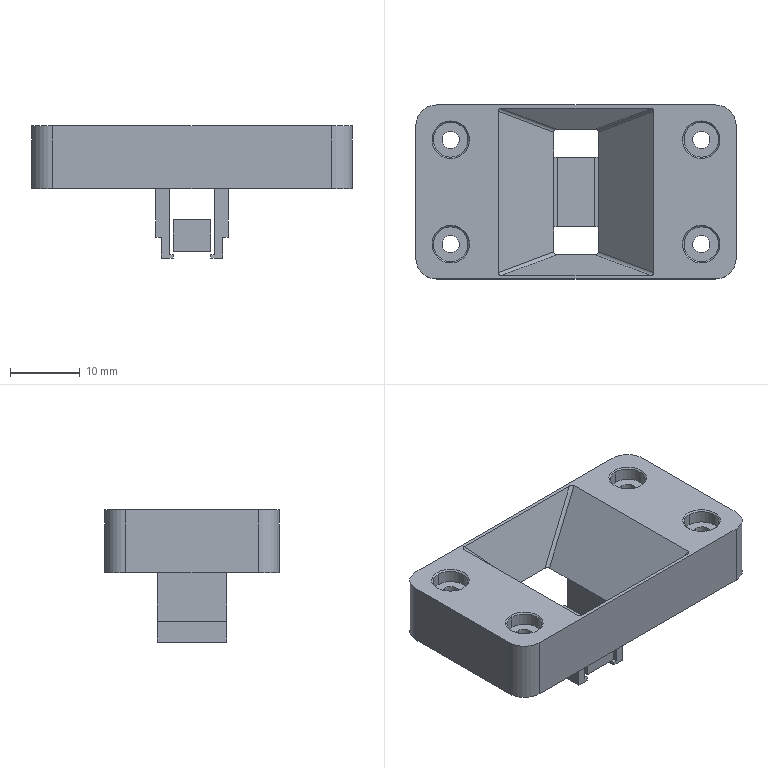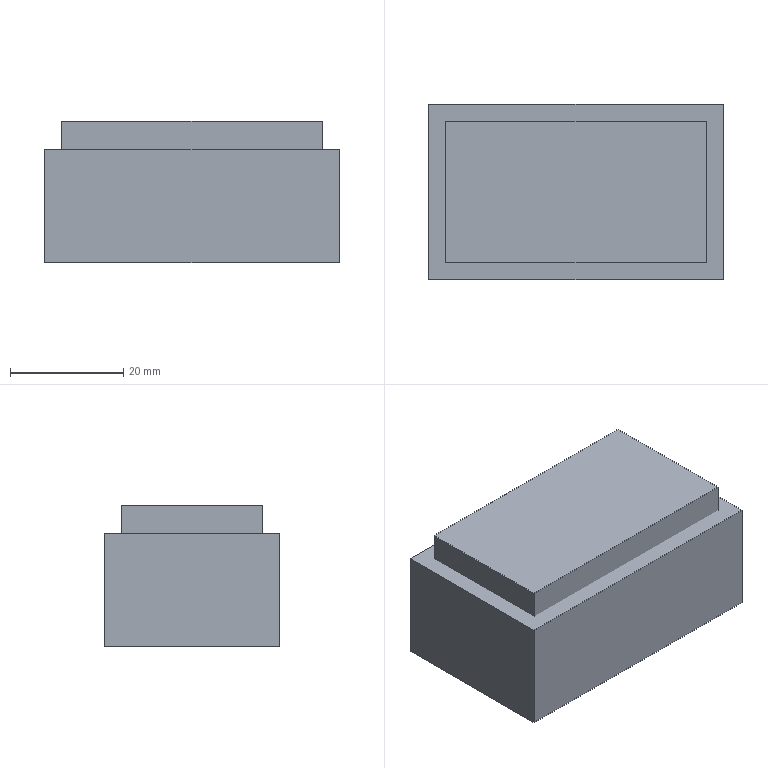CAM job | NX | 3-axis milling, drilling | part box 46 x 25 x 19 mm | stock box 52 x 31 x 25 mm
Tools:
number,name,description,diameter,corner_radius,flute_length,length,flutes
1,D63,Milling Tool-5 Parameters,63.0,0.0,50.0,75.0,2
7,D6A45,Milling Tool-5 Parameters,6.0,0.0,3.0,3.0,2
12,2.5ZT,Drilling Tool,2.5,0.0,35.0,50.0,2
10,D10,Milling Tool-5 Parameters,10.0,0.0,50.0,75.0,2
11,D10JING,Milling Tool-5 Parameters,10.0,0.0,50.0,75.0,2
3,D3,Milling Tool-5 Parameters,3.0,0.0,50.0,75.0,2
6,D6,Milling Tool-5 Parameters,6.0,0.0,50.0,75.0,2
4,D4,Milling Tool-5 Parameters,4.0,0.0,50.0,75.0,2
5,D2R0.2,Milling Tool-5 Parameters,2.0,0.2,50.0,75.0,2
Operations:
program,operation,operation_type,tool,method,geometry_group,spindle_rpm,surface_speed,feed_per_tooth,feed_cut,feed_plunge,cut_length_mm,path_length_mm,cut_time_min,machine_time_min
1,FLOOR_WALL,VolumeBased25DMillingOperation,D63,METHOD,A,6500.0,1286.0,0.0962,1250.0,100.0,127.0,181.0,0.1016,0.107
1,DRILLING_COPY_1,Operation,D6A45,METHOD,A,5000.0,94.0,0.025,250.0,0.0,16.0,167.719,0.064,0.0792
1,DRILLING_COPY_COPY_1,Operation,2.5ZT,METHOD,A,2000.0,15.0,0.03,120.0,0.0,57.004,252.718,0.475,0.4946
1,ADAPTIVE_MILLING,CavityMilling,D10,METHOD,A,9500.0,298.0,0.1579,3000.0,1000.0,710.321,804.321,0.2374,0.2468
1,ZLEVEL_PROFILE_COPY_COPY_1,ZLevelMilling,D10JING,METHOD,A,9500.0,298.0,0.0632,1200.0,100.0,176.311,268.311,0.1469,0.1561
1,FIXED_CONTOUR,SurfaceContour,D6,METHOD,A,9500.0,179.0,0.1316,2500.0,500.0,1874.519,1934.519,0.7559,0.7619
1,ZLEVEL_PROFILE,ZLevelMilling,D4,METHOD,A,9500.0,119.0,0.1053,2000.0,800.0,1329.602,1414.602,0.6899,0.6984
1,ZLEVEL_PROFILE_COPY,ZLevelMilling,D4,METHOD,A,9500.0,119.0,0.0632,1200.0,800.0,255.121,339.621,0.2397,0.2481
1,ZLEVEL_PROFILE_COPY_COPY,ZLevelMilling,D4,METHOD,A,9500.0,119.0,0.0632,1200.0,800.0,73.016,167.517,0.0768,0.0862
1,HOLE_MILLING,CylinderMilling,D3,METHOD,A,9500.0,89.0,0.0658,1250.0,100.0,222.69,534.69,0.1782,0.2094
1,FIXED_CONTOUR_COPY,SurfaceContour,D2R0.2,METHOD,A,9500.0,59.0,0.1316,2500.0,500.0,10231.215,10422.764,4.138,4.157
1,ZLEVEL_PROFILE_1_COPY_1,ZLevelMilling,D6A45,METHOD,A,9500.0,179.0,0.0526,1000.0,100.0,212.818,667.365,0.2128,0.2583
1,刀补3,CylinderMilling,D3,METHOD,A,9500.0,89.0,0.0579,1100.0,100.0,96.418,408.418,0.0877,0.1189
2,FLOOR_WALL_COPY,VolumeBased25DMillingOperation,D63,METHOD,B,6500.0,1286.0,0.0962,1250.0,100.0,726.0,1595.002,0.5808,0.6677
2,ADAPTIVE_MILLING_COPY,CavityMilling,D10,METHOD,B,9500.0,298.0,0.1579,3000.0,1000.0,1704.845,1925.66,0.5703,0.5924
2,FLOOR_WALL_1,VolumeBased25DMillingOperation,D6,METHOD,B,9500.0,179.0,0.0658,1250.0,100.0,680.48,1353.624,0.5444,0.6117
2,ZLEVEL_PROFILE_1_COPY_1_COPY,ZLevelMilling,D6A45,METHOD,B,9500.0,179.0,0.0526,1000.0,100.0,69.012,198.976,0.069,0.082
2,ZLEVEL_PROFILE_1_COPY_1_COPY_COPY,ZLevelMilling,D6A45,METHOD,B,9500.0,179.0,0.0526,1000.0,100.0,168.679,697.281,0.1687,0.2215